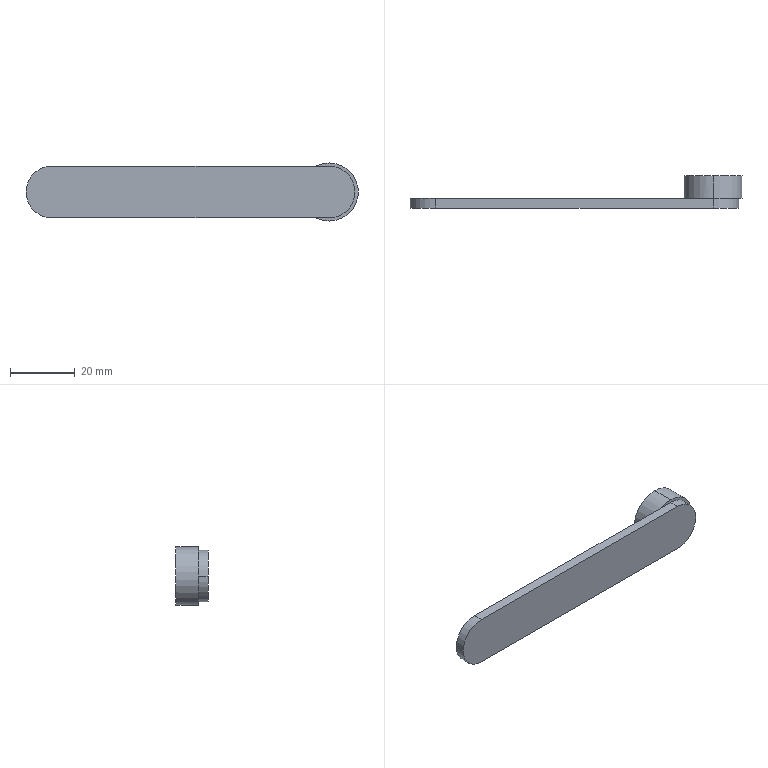Part | STEP file | 开关-3 | 1 solid | 12 faces | box 103 x 10 x 18 mm | volume 6512 mm3 | cylinder 6 | plane 6 | commonest cylinder face diameters 16 x4 18 x2
STEP:
#1=CARTESIAN_POINT('',(0.,0.,0.));
#2=DIRECTION('',(0.,0.,1.));
#3=DIRECTION('',(1.,0.,0.));
#4=AXIS2_PLACEMENT_3D('',#1,#2,#3);
#5=CARTESIAN_POINT('',(43.,10.,9.));
#6=VERTEX_POINT('',#5);
#7=CARTESIAN_POINT('',(43.,10.,-9.));
#8=VERTEX_POINT('',#7);
#9=CARTESIAN_POINT('',(43.,10.,0.));
#10=DIRECTION('',(0.,1.,0.));
#11=DIRECTION('',(0.,0.,1.));
#12=AXIS2_PLACEMENT_3D('',#9,#10,#11);
#13=CIRCLE('',#12,9.);
#14=CARTESIAN_POINT('',(43.,10.,0.));
#15=DIRECTION('',(0.,-1.,0.));
#16=DIRECTION('',(0.,0.,-1.));
#17=AXIS2_PLACEMENT_3D('',#14,#15,#16);
#18=CYLINDRICAL_SURFACE('',#17,9.);
#19=CARTESIAN_POINT('',(3.142,0.));
#20=DIRECTION('',(-1.,0.));
#21=VECTOR('',#20,1.);
#22=LINE('',#19,#21);
#23=(GEOMETRIC_REPRESENTATION_CONTEXT(2)PARAMETRIC_REPRESENTATION_CONTEXT()REPRESENTATION_CONTEXT('',''));
#24=DEFINITIONAL_REPRESENTATION('',(#22),#23);
#25=PCURVE('',#18,#24);
#26=CARTESIAN_POINT('',(43.,10.,0.));
#27=DIRECTION('',(0.,1.,0.));
#28=DIRECTION('',(0.,0.,1.));
#29=AXIS2_PLACEMENT_3D('',#26,#27,#28);
#30=PLANE('',#29);
#31=CARTESIAN_POINT('',(0.,0.));
#32=DIRECTION('',(1.,0.));
#33=AXIS2_PLACEMENT_2D('',#31,#32);
#34=CIRCLE('',#33,9.);
#35=(GEOMETRIC_REPRESENTATION_CONTEXT(2)PARAMETRIC_REPRESENTATION_CONTEXT()REPRESENTATION_CONTEXT('',''));
#36=DEFINITIONAL_REPRESENTATION('',(#34),#35);
#37=PCURVE('',#30,#36);
#38=SURFACE_CURVE('',#13,(#25,#37),.PCURVE_S1.);
#39=EDGE_CURVE('',#6,#8,#38,.T.);
#40=ORIENTED_EDGE('',*,*,#39,.F.);
#41=CARTESIAN_POINT('',(43.,3.,9.));
#42=VERTEX_POINT('',#41);
#43=CARTESIAN_POINT('',(43.,10.,9.));
#44=DIRECTION('',(0.,-1.,0.));
#45=VECTOR('',#44,1.);
#46=LINE('',#43,#45);
#47=CARTESIAN_POINT('',(3.142,0.));
#48=DIRECTION('',(0.,1.));
#49=VECTOR('',#48,1.);
#50=LINE('',#47,#49);
#51=(GEOMETRIC_REPRESENTATION_CONTEXT(2)PARAMETRIC_REPRESENTATION_CONTEXT()REPRESENTATION_CONTEXT('',''));
#52=DEFINITIONAL_REPRESENTATION('',(#50),#51);
#53=PCURVE('',#18,#52);
#54=CARTESIAN_POINT('',(43.,10.,0.));
#55=DIRECTION('',(0.,-1.,0.));
#56=DIRECTION('',(0.,0.,-1.));
#57=AXIS2_PLACEMENT_3D('',#54,#55,#56);
#58=CYLINDRICAL_SURFACE('',#57,9.);
#59=CARTESIAN_POINT('',(3.142,0.));
#60=DIRECTION('',(0.,1.));
#61=VECTOR('',#60,1.);
#62=LINE('',#59,#61);
#63=(GEOMETRIC_REPRESENTATION_CONTEXT(2)PARAMETRIC_REPRESENTATION_CONTEXT()REPRESENTATION_CONTEXT('',''));
#64=DEFINITIONAL_REPRESENTATION('',(#62),#63);
#65=PCURVE('',#58,#64);
#66=SURFACE_CURVE('',#46,(#53,#65),.PCURVE_S1.);
#67=EDGE_CURVE('',#6,#42,#66,.T.);
#68=ORIENTED_EDGE('',*,*,#67,.T.);
#69=CARTESIAN_POINT('',(43.,3.,-9.));
#70=VERTEX_POINT('',#69);
#71=CARTESIAN_POINT('',(43.,3.,0.));
#72=DIRECTION('',(0.,1.,0.));
#73=DIRECTION('',(0.,0.,1.));
#74=AXIS2_PLACEMENT_3D('',#71,#72,#73);
#75=CIRCLE('',#74,9.);
#76=CARTESIAN_POINT('',(3.142,7.));
#77=DIRECTION('',(-1.,0.));
#78=VECTOR('',#77,1.);
#79=LINE('',#76,#78);
#80=(GEOMETRIC_REPRESENTATION_CONTEXT(2)PARAMETRIC_REPRESENTATION_CONTEXT()REPRESENTATION_CONTEXT('',''));
#81=DEFINITIONAL_REPRESENTATION('',(#79),#80);
#82=PCURVE('',#18,#81);
#83=CARTESIAN_POINT('',(43.,3.,0.));
#84=DIRECTION('',(0.,1.,0.));
#85=DIRECTION('',(0.,0.,1.));
#86=AXIS2_PLACEMENT_3D('',#83,#84,#85);
#87=PLANE('',#86);
#88=CARTESIAN_POINT('',(0.,0.));
#89=DIRECTION('',(1.,0.));
#90=AXIS2_PLACEMENT_2D('',#88,#89);
#91=CIRCLE('',#90,9.);
#92=(GEOMETRIC_REPRESENTATION_CONTEXT(2)PARAMETRIC_REPRESENTATION_CONTEXT()REPRESENTATION_CONTEXT('',''));
#93=DEFINITIONAL_REPRESENTATION('',(#91),#92);
#94=PCURVE('',#87,#93);
#95=SURFACE_CURVE('',#75,(#82,#94),.PCURVE_S1.);
#96=EDGE_CURVE('',#42,#70,#95,.T.);
#97=ORIENTED_EDGE('',*,*,#96,.T.);
#98=CARTESIAN_POINT('',(43.,10.,-9.));
#99=DIRECTION('',(0.,-1.,0.));
#100=VECTOR('',#99,1.);
#101=LINE('',#98,#100);
#102=CARTESIAN_POINT('',(0.,0.));
#103=DIRECTION('',(0.,1.));
#104=VECTOR('',#103,1.);
#105=LINE('',#102,#104);
#106=(GEOMETRIC_REPRESENTATION_CONTEXT(2)PARAMETRIC_REPRESENTATION_CONTEXT()REPRESENTATION_CONTEXT('',''));
#107=DEFINITIONAL_REPRESENTATION('',(#105),#106);
#108=PCURVE('',#18,#107);
#109=CARTESIAN_POINT('',(6.283,0.));
#110=DIRECTION('',(0.,1.));
#111=VECTOR('',#110,1.);
#112=LINE('',#109,#111);
#113=(GEOMETRIC_REPRESENTATION_CONTEXT(2)PARAMETRIC_REPRESENTATION_CONTEXT()REPRESENTATION_CONTEXT('',''));
#114=DEFINITIONAL_REPRESENTATION('',(#112),#113);
#115=PCURVE('',#58,#114);
#116=SURFACE_CURVE('',#101,(#108,#115),.PCURVE_S1.);
#117=EDGE_CURVE('',#8,#70,#116,.T.);
#118=ORIENTED_EDGE('',*,*,#117,.F.);
#119=EDGE_LOOP('',(#40,#68,#97,#118));
#120=FACE_BOUND('',#119,.T.);
#121=ADVANCED_FACE('',(#120),#18,.T.);
#122=CARTESIAN_POINT('',(43.,0.,-8.));
#123=VERTEX_POINT('',#122);
#124=CARTESIAN_POINT('',(-43.,0.,-8.));
#125=VERTEX_POINT('',#124);
#126=CARTESIAN_POINT('',(-51.,0.,-8.));
#127=DIRECTION('',(-1.,0.,0.));
#128=VECTOR('',#127,1.);
#129=LINE('',#126,#128);
#130=CARTESIAN_POINT('',(-51.,3.,-8.));
#131=DIRECTION('',(0.,0.,1.));
#132=DIRECTION('',(1.,0.,0.));
#133=AXIS2_PLACEMENT_3D('',#130,#131,#132);
#134=PLANE('',#133);
#135=CARTESIAN_POINT('',(0.,-3.));
#136=DIRECTION('',(-1.,0.));
#137=VECTOR('',#136,1.);
#138=LINE('',#135,#137);
#139=(GEOMETRIC_REPRESENTATION_CONTEXT(2)PARAMETRIC_REPRESENTATION_CONTEXT()REPRESENTATION_CONTEXT('',''));
#140=DEFINITIONAL_REPRESENTATION('',(#138),#139);
#141=PCURVE('',#134,#140);
#142=CARTESIAN_POINT('',(0.,0.,0.));
#143=DIRECTION('',(0.,-1.,0.));
#144=DIRECTION('',(0.,0.,-1.));
#145=AXIS2_PLACEMENT_3D('',#142,#143,#144);
#146=PLANE('',#145);
#147=CARTESIAN_POINT('',(8.,-51.));
#148=DIRECTION('',(0.,-1.));
#149=VECTOR('',#148,1.);
#150=LINE('',#147,#149);
#151=(GEOMETRIC_REPRESENTATION_CONTEXT(2)PARAMETRIC_REPRESENTATION_CONTEXT()REPRESENTATION_CONTEXT('',''));
#152=DEFINITIONAL_REPRESENTATION('',(#150),#151);
#153=PCURVE('',#146,#152);
#154=SURFACE_CURVE('',#129,(#141,#153),.PCURVE_S1.);
#155=EDGE_CURVE('',#123,#125,#154,.T.);
#156=ORIENTED_EDGE('',*,*,#155,.T.);
#157=CARTESIAN_POINT('',(-43.,3.,-8.));
#158=VERTEX_POINT('',#157);
#159=CARTESIAN_POINT('',(-43.,3.,-8.));
#160=DIRECTION('',(0.,1.,0.));
#161=VECTOR('',#160,1.);
#162=LINE('',#159,#161);
#163=CARTESIAN_POINT('',(8.,0.));
#164=DIRECTION('',(0.,1.));
#165=VECTOR('',#164,1.);
#166=LINE('',#163,#165);
#167=(GEOMETRIC_REPRESENTATION_CONTEXT(2)PARAMETRIC_REPRESENTATION_CONTEXT()REPRESENTATION_CONTEXT('',''));
#168=DEFINITIONAL_REPRESENTATION('',(#166),#167);
#169=PCURVE('',#134,#168);
#170=CARTESIAN_POINT('',(-43.,3.,0.));
#171=DIRECTION('',(0.,-1.,0.));
#172=DIRECTION('',(0.,0.,-1.));
#173=AXIS2_PLACEMENT_3D('',#170,#171,#172);
#174=CYLINDRICAL_SURFACE('',#173,8.);
#175=CARTESIAN_POINT('',(6.283,0.));
#176=DIRECTION('',(0.,-1.));
#177=VECTOR('',#176,1.);
#178=LINE('',#175,#177);
#179=(GEOMETRIC_REPRESENTATION_CONTEXT(2)PARAMETRIC_REPRESENTATION_CONTEXT()REPRESENTATION_CONTEXT('',''));
#180=DEFINITIONAL_REPRESENTATION('',(#178),#179);
#181=PCURVE('',#174,#180);
#182=SURFACE_CURVE('',#162,(#169,#181),.PCURVE_S1.);
#183=EDGE_CURVE('',#125,#158,#182,.T.);
#184=ORIENTED_EDGE('',*,*,#183,.T.);
#185=CARTESIAN_POINT('',(38.877,3.,-8.));
#186=VERTEX_POINT('',#185);
#187=CARTESIAN_POINT('',(-51.,3.,-8.));
#188=DIRECTION('',(-1.,0.,0.));
#189=VECTOR('',#188,1.);
#190=LINE('',#187,#189);
#191=CARTESIAN_POINT('',(0.,0.));
#192=DIRECTION('',(-1.,0.));
#193=VECTOR('',#192,1.);
#194=LINE('',#191,#193);
#195=(GEOMETRIC_REPRESENTATION_CONTEXT(2)PARAMETRIC_REPRESENTATION_CONTEXT()REPRESENTATION_CONTEXT('',''));
#196=DEFINITIONAL_REPRESENTATION('',(#194),#195);
#197=PCURVE('',#134,#196);
#198=CARTESIAN_POINT('',(0.,3.,0.));
#199=DIRECTION('',(0.,-1.,0.));
#200=DIRECTION('',(0.,0.,-1.));
#201=AXIS2_PLACEMENT_3D('',#198,#199,#200);
#202=PLANE('',#201);
#203=CARTESIAN_POINT('',(8.,-51.));
#204=DIRECTION('',(0.,-1.));
#205=VECTOR('',#204,1.);
#206=LINE('',#203,#205);
#207=(GEOMETRIC_REPRESENTATION_CONTEXT(2)PARAMETRIC_REPRESENTATION_CONTEXT()REPRESENTATION_CONTEXT('',''));
#208=DEFINITIONAL_REPRESENTATION('',(#206),#207);
#209=PCURVE('',#202,#208);
#210=SURFACE_CURVE('',#190,(#197,#209),.PCURVE_S1.);
#211=EDGE_CURVE('',#186,#158,#210,.T.);
#212=ORIENTED_EDGE('',*,*,#211,.F.);
#213=CARTESIAN_POINT('',(43.,3.,-8.));
#214=VERTEX_POINT('',#213);
#215=CARTESIAN_POINT('',(-51.,3.,-8.));
#216=DIRECTION('',(-1.,0.,0.));
#217=VECTOR('',#216,1.);
#218=LINE('',#215,#217);
#219=CARTESIAN_POINT('',(0.,0.));
#220=DIRECTION('',(-1.,0.));
#221=VECTOR('',#220,1.);
#222=LINE('',#219,#221);
#223=(GEOMETRIC_REPRESENTATION_CONTEXT(2)PARAMETRIC_REPRESENTATION_CONTEXT()REPRESENTATION_CONTEXT('',''));
#224=DEFINITIONAL_REPRESENTATION('',(#222),#223);
#225=PCURVE('',#134,#224);
#226=CARTESIAN_POINT('',(-8.,-94.));
#227=DIRECTION('',(0.,-1.));
#228=VECTOR('',#227,1.);
#229=LINE('',#226,#228);
#230=(GEOMETRIC_REPRESENTATION_CONTEXT(2)PARAMETRIC_REPRESENTATION_CONTEXT()REPRESENTATION_CONTEXT('',''));
#231=DEFINITIONAL_REPRESENTATION('',(#229),#230);
#232=PCURVE('',#87,#231);
#233=SURFACE_CURVE('',#218,(#225,#232),.PCURVE_S1.);
#234=EDGE_CURVE('',#214,#186,#233,.T.);
#235=ORIENTED_EDGE('',*,*,#234,.F.);
#236=CARTESIAN_POINT('',(43.,3.,-8.));
#237=DIRECTION('',(0.,-1.,0.));
#238=VECTOR('',#237,1.);
#239=LINE('',#236,#238);
#240=CARTESIAN_POINT('',(94.,0.));
#241=DIRECTION('',(0.,-1.));
#242=VECTOR('',#241,1.);
#243=LINE('',#240,#242);
#244=(GEOMETRIC_REPRESENTATION_CONTEXT(2)PARAMETRIC_REPRESENTATION_CONTEXT()REPRESENTATION_CONTEXT('',''));
#245=DEFINITIONAL_REPRESENTATION('',(#243),#244);
#246=PCURVE('',#134,#245);
#247=CARTESIAN_POINT('',(43.,3.,0.));
#248=DIRECTION('',(0.,-1.,0.));
#249=DIRECTION('',(0.,0.,-1.));
#250=AXIS2_PLACEMENT_3D('',#247,#248,#249);
#251=CYLINDRICAL_SURFACE('',#250,8.);
#252=CARTESIAN_POINT('',(0.,0.));
#253=DIRECTION('',(0.,1.));
#254=VECTOR('',#253,1.);
#255=LINE('',#252,#254);
#256=(GEOMETRIC_REPRESENTATION_CONTEXT(2)PARAMETRIC_REPRESENTATION_CONTEXT()REPRESENTATION_CONTEXT('',''));
#257=DEFINITIONAL_REPRESENTATION('',(#255),#256);
#258=PCURVE('',#251,#257);
#259=SURFACE_CURVE('',#239,(#246,#258),.PCURVE_S1.);
#260=EDGE_CURVE('',#214,#123,#259,.T.);
#261=ORIENTED_EDGE('',*,*,#260,.T.);
#262=EDGE_LOOP('',(#156,#184,#212,#235,#261));
#263=FACE_BOUND('',#262,.T.);
#264=ADVANCED_FACE('',(#263),#134,.F.);
#265=CARTESIAN_POINT('',(-43.,3.,8.));
#266=VERTEX_POINT('',#265);
#267=CARTESIAN_POINT('',(38.877,3.,8.));
#268=VERTEX_POINT('',#267);
#269=CARTESIAN_POINT('',(-51.,3.,8.));
#270=DIRECTION('',(1.,0.,0.));
#271=VECTOR('',#270,1.);
#272=LINE('',#269,#271);
#273=CARTESIAN_POINT('',(-51.,3.,8.));
#274=DIRECTION('',(0.,0.,-1.));
#275=DIRECTION('',(-1.,0.,0.));
#276=AXIS2_PLACEMENT_3D('',#273,#274,#275);
#277=PLANE('',#276);
#278=CARTESIAN_POINT('',(0.,0.));
#279=DIRECTION('',(-1.,0.));
#280=VECTOR('',#279,1.);
#281=LINE('',#278,#280);
#282=(GEOMETRIC_REPRESENTATION_CONTEXT(2)PARAMETRIC_REPRESENTATION_CONTEXT()REPRESENTATION_CONTEXT('',''));
#283=DEFINITIONAL_REPRESENTATION('',(#281),#282);
#284=PCURVE('',#277,#283);
#285=CARTESIAN_POINT('',(-8.,-51.));
#286=DIRECTION('',(0.,1.));
#287=VECTOR('',#286,1.);
#288=LINE('',#285,#287);
#289=(GEOMETRIC_REPRESENTATION_CONTEXT(2)PARAMETRIC_REPRESENTATION_CONTEXT()REPRESENTATION_CONTEXT('',''));
#290=DEFINITIONAL_REPRESENTATION('',(#288),#289);
#291=PCURVE('',#202,#290);
#292=SURFACE_CURVE('',#272,(#284,#291),.PCURVE_S1.);
#293=EDGE_CURVE('',#266,#268,#292,.T.);
#294=ORIENTED_EDGE('',*,*,#293,.F.);
#295=CARTESIAN_POINT('',(-43.,0.,8.));
#296=VERTEX_POINT('',#295);
#297=CARTESIAN_POINT('',(-43.,3.,8.));
#298=DIRECTION('',(0.,-1.,0.));
#299=VECTOR('',#298,1.);
#300=LINE('',#297,#299);
#301=CARTESIAN_POINT('',(-8.,0.));
#302=DIRECTION('',(0.,-1.));
#303=VECTOR('',#302,1.);
#304=LINE('',#301,#303);
#305=(GEOMETRIC_REPRESENTATION_CONTEXT(2)PARAMETRIC_REPRESENTATION_CONTEXT()REPRESENTATION_CONTEXT('',''));
#306=DEFINITIONAL_REPRESENTATION('',(#304),#305);
#307=PCURVE('',#277,#306);
#308=CARTESIAN_POINT('',(-43.,3.,0.));
#309=DIRECTION('',(0.,-1.,0.));
#310=DIRECTION('',(0.,0.,-1.));
#311=AXIS2_PLACEMENT_3D('',#308,#309,#310);
#312=CYLINDRICAL_SURFACE('',#311,8.);
#313=CARTESIAN_POINT('',(3.142,0.));
#314=DIRECTION('',(0.,1.));
#315=VECTOR('',#314,1.);
#316=LINE('',#313,#315);
#317=(GEOMETRIC_REPRESENTATION_CONTEXT(2)PARAMETRIC_REPRESENTATION_CONTEXT()REPRESENTATION_CONTEXT('',''));
#318=DEFINITIONAL_REPRESENTATION('',(#316),#317);
#319=PCURVE('',#312,#318);
#320=SURFACE_CURVE('',#300,(#307,#319),.PCURVE_S1.);
#321=EDGE_CURVE('',#266,#296,#320,.T.);
#322=ORIENTED_EDGE('',*,*,#321,.T.);
#323=CARTESIAN_POINT('',(43.,0.,8.));
#324=VERTEX_POINT('',#323);
#325=CARTESIAN_POINT('',(-51.,0.,8.));
#326=DIRECTION('',(1.,0.,0.));
#327=VECTOR('',#326,1.);
#328=LINE('',#325,#327);
#329=CARTESIAN_POINT('',(0.,-3.));
#330=DIRECTION('',(-1.,0.));
#331=VECTOR('',#330,1.);
#332=LINE('',#329,#331);
#333=(GEOMETRIC_REPRESENTATION_CONTEXT(2)PARAMETRIC_REPRESENTATION_CONTEXT()REPRESENTATION_CONTEXT('',''));
#334=DEFINITIONAL_REPRESENTATION('',(#332),#333);
#335=PCURVE('',#277,#334);
#336=CARTESIAN_POINT('',(-8.,-51.));
#337=DIRECTION('',(0.,1.));
#338=VECTOR('',#337,1.);
#339=LINE('',#336,#338);
#340=(GEOMETRIC_REPRESENTATION_CONTEXT(2)PARAMETRIC_REPRESENTATION_CONTEXT()REPRESENTATION_CONTEXT('',''));
#341=DEFINITIONAL_REPRESENTATION('',(#339),#340);
#342=PCURVE('',#146,#341);
#343=SURFACE_CURVE('',#328,(#335,#342),.PCURVE_S1.);
#344=EDGE_CURVE('',#296,#324,#343,.T.);
#345=ORIENTED_EDGE('',*,*,#344,.T.);
#346=CARTESIAN_POINT('',(43.,3.,8.));
#347=VERTEX_POINT('',#346);
#348=CARTESIAN_POINT('',(43.,3.,8.));
#349=DIRECTION('',(0.,1.,0.));
#350=VECTOR('',#349,1.);
#351=LINE('',#348,#350);
#352=CARTESIAN_POINT('',(-94.,0.));
#353=DIRECTION('',(0.,1.));
#354=VECTOR('',#353,1.);
#355=LINE('',#352,#354);
#356=(GEOMETRIC_REPRESENTATION_CONTEXT(2)PARAMETRIC_REPRESENTATION_CONTEXT()REPRESENTATION_CONTEXT('',''));
#357=DEFINITIONAL_REPRESENTATION('',(#355),#356);
#358=PCURVE('',#277,#357);
#359=CARTESIAN_POINT('',(43.,3.,0.));
#360=DIRECTION('',(0.,-1.,0.));
#361=DIRECTION('',(0.,0.,-1.));
#362=AXIS2_PLACEMENT_3D('',#359,#360,#361);
#363=CYLINDRICAL_SURFACE('',#362,8.);
#364=CARTESIAN_POINT('',(3.142,0.));
#365=DIRECTION('',(0.,-1.));
#366=VECTOR('',#365,1.);
#367=LINE('',#364,#366);
#368=(GEOMETRIC_REPRESENTATION_CONTEXT(2)PARAMETRIC_REPRESENTATION_CONTEXT()REPRESENTATION_CONTEXT('',''));
#369=DEFINITIONAL_REPRESENTATION('',(#367),#368);
#370=PCURVE('',#363,#369);
#371=SURFACE_CURVE('',#351,(#358,#370),.PCURVE_S1.);
#372=EDGE_CURVE('',#324,#347,#371,.T.);
#373=ORIENTED_EDGE('',*,*,#372,.T.);
#374=CARTESIAN_POINT('',(-51.,3.,8.));
#375=DIRECTION('',(1.,0.,0.));
#376=VECTOR('',#375,1.);
#377=LINE('',#374,#376);
#378=CARTESIAN_POINT('',(0.,0.));
#379=DIRECTION('',(-1.,0.));
#380=VECTOR('',#379,1.);
#381=LINE('',#378,#380);
#382=(GEOMETRIC_REPRESENTATION_CONTEXT(2)PARAMETRIC_REPRESENTATION_CONTEXT()REPRESENTATION_CONTEXT('',''));
#383=DEFINITIONAL_REPRESENTATION('',(#381),#382);
#384=PCURVE('',#277,#383);
#385=CARTESIAN_POINT('',(8.,-94.));
#386=DIRECTION('',(0.,1.));
#387=VECTOR('',#386,1.);
#388=LINE('',#385,#387);
#389=(GEOMETRIC_REPRESENTATION_CONTEXT(2)PARAMETRIC_REPRESENTATION_CONTEXT()REPRESENTATION_CONTEXT('',''));
#390=DEFINITIONAL_REPRESENTATION('',(#388),#389);
#391=PCURVE('',#87,#390);
#392=SURFACE_CURVE('',#377,(#384,#391),.PCURVE_S1.);
#393=EDGE_CURVE('',#268,#347,#392,.T.);
#394=ORIENTED_EDGE('',*,*,#393,.F.);
#395=EDGE_LOOP('',(#294,#322,#345,#373,#394));
#396=FACE_BOUND('',#395,.T.);
#397=ADVANCED_FACE('',(#396),#277,.F.);
#398=CARTESIAN_POINT('',(43.,3.,0.));
#399=DIRECTION('',(0.,1.,0.));
#400=DIRECTION('',(0.,0.,1.));
#401=AXIS2_PLACEMENT_3D('',#398,#399,#400);
#402=CIRCLE('',#401,9.);
#403=CARTESIAN_POINT('',(-9.,43.));
#404=CARTESIAN_POINT('',(-9.,58.588));
#405=CARTESIAN_POINT('',(4.5,50.794));
#406=CARTESIAN_POINT('',(18.,43.));
#407=CARTESIAN_POINT('',(4.5,35.206));
#408=CARTESIAN_POINT('',(-9.,27.412));
#409=CARTESIAN_POINT('',(-9.,43.));
#410=(BOUNDED_CURVE()B_SPLINE_CURVE(2,(#403,#404,#405,#406,#407,#408,#409),.UNSPECIFIED.,.T.,.F.)B_SPLINE_CURVE_WITH_KNOTS((1,2,2,2,2,1),(-2.094,0.,2.094,4.189,6.283,8.378),.UNSPECIFIED.)CURVE()GEOMETRIC_REPRESENTATION_ITEM()RATIONAL_B_SPLINE_CURVE((1.,0.5,1.,0.5,1.,0.5,1.))REPRESENTATION_ITEM(''));
#411=(GEOMETRIC_REPRESENTATION_CONTEXT(2)PARAMETRIC_REPRESENTATION_CONTEXT()REPRESENTATION_CONTEXT('',''));
#412=DEFINITIONAL_REPRESENTATION('',(#410),#411);
#413=PCURVE('',#202,#412);
#414=CARTESIAN_POINT('',(9.425,7.));
#415=DIRECTION('',(-1.,0.));
#416=VECTOR('',#415,1.);
#417=LINE('',#414,#416);
#418=(GEOMETRIC_REPRESENTATION_CONTEXT(2)PARAMETRIC_REPRESENTATION_CONTEXT()REPRESENTATION_CONTEXT('',''));
#419=DEFINITIONAL_REPRESENTATION('',(#417),#418);
#420=PCURVE('',#58,#419);
#421=SURFACE_CURVE('',#402,(#413,#420),.PCURVE_S1.);
#422=EDGE_CURVE('',#186,#268,#421,.T.);
#423=ORIENTED_EDGE('',*,*,#422,.F.);
#424=ORIENTED_EDGE('',*,*,#211,.T.);
#425=CARTESIAN_POINT('',(-51.,3.,0.));
#426=VERTEX_POINT('',#425);
#427=CARTESIAN_POINT('',(-43.,3.,0.));
#428=DIRECTION('',(0.,1.,0.));
#429=DIRECTION('',(0.,0.,-1.));
#430=AXIS2_PLACEMENT_3D('',#427,#428,#429);
#431=CIRCLE('',#430,8.);
#432=CARTESIAN_POINT('',(8.,-43.));
#433=CARTESIAN_POINT('',(8.,-56.856));
#434=CARTESIAN_POINT('',(-4.,-49.928));
#435=CARTESIAN_POINT('',(-16.,-43.));
#436=CARTESIAN_POINT('',(-4.,-36.072));
#437=CARTESIAN_POINT('',(8.,-29.144));
#438=CARTESIAN_POINT('',(8.,-43.));
#439=(BOUNDED_CURVE()B_SPLINE_CURVE(2,(#432,#433,#434,#435,#436,#437,#438),.UNSPECIFIED.,.T.,.F.)B_SPLINE_CURVE_WITH_KNOTS((1,2,2,2,2,1),(-2.094,0.,2.094,4.189,6.283,8.378),.UNSPECIFIED.)CURVE()GEOMETRIC_REPRESENTATION_ITEM()RATIONAL_B_SPLINE_CURVE((1.,0.5,1.,0.5,1.,0.5,1.))REPRESENTATION_ITEM(''));
#440=(GEOMETRIC_REPRESENTATION_CONTEXT(2)PARAMETRIC_REPRESENTATION_CONTEXT()REPRESENTATION_CONTEXT('',''));
#441=DEFINITIONAL_REPRESENTATION('',(#439),#440);
#442=PCURVE('',#202,#441);
#443=CARTESIAN_POINT('',(6.283,0.));
#444=DIRECTION('',(-1.,0.));
#445=VECTOR('',#444,1.);
#446=LINE('',#443,#445);
#447=(GEOMETRIC_REPRESENTATION_CONTEXT(2)PARAMETRIC_REPRESENTATION_CONTEXT()REPRESENTATION_CONTEXT('',''));
#448=DEFINITIONAL_REPRESENTATION('',(#446),#447);
#449=PCURVE('',#174,#448);
#450=SURFACE_CURVE('',#431,(#442,#449),.PCURVE_S1.);
#451=EDGE_CURVE('',#158,#426,#450,.T.);
#452=ORIENTED_EDGE('',*,*,#451,.T.);
#453=CARTESIAN_POINT('',(-43.,3.,0.));
#454=DIRECTION('',(0.,1.,0.));
#455=DIRECTION('',(0.,0.,-1.));
#456=AXIS2_PLACEMENT_3D('',#453,#454,#455);
#457=CIRCLE('',#456,8.);
#458=CARTESIAN_POINT('',(8.,-43.));
#459=CARTESIAN_POINT('',(8.,-56.856));
#460=CARTESIAN_POINT('',(-4.,-49.928));
#461=CARTESIAN_POINT('',(-16.,-43.));
#462=CARTESIAN_POINT('',(-4.,-36.072));
#463=CARTESIAN_POINT('',(8.,-29.144));
#464=CARTESIAN_POINT('',(8.,-43.));
#465=(BOUNDED_CURVE()B_SPLINE_CURVE(2,(#458,#459,#460,#461,#462,#463,#464),.UNSPECIFIED.,.T.,.F.)B_SPLINE_CURVE_WITH_KNOTS((1,2,2,2,2,1),(-2.094,0.,2.094,4.189,6.283,8.378),.UNSPECIFIED.)CURVE()GEOMETRIC_REPRESENTATION_ITEM()RATIONAL_B_SPLINE_CURVE((1.,0.5,1.,0.5,1.,0.5,1.))REPRESENTATION_ITEM(''));
#466=(GEOMETRIC_REPRESENTATION_CONTEXT(2)PARAMETRIC_REPRESENTATION_CONTEXT()REPRESENTATION_CONTEXT('',''));
#467=DEFINITIONAL_REPRESENTATION('',(#465),#466);
#468=PCURVE('',#202,#467);
#469=CARTESIAN_POINT('',(6.283,0.));
#470=DIRECTION('',(-1.,0.));
#471=VECTOR('',#470,1.);
#472=LINE('',#469,#471);
#473=(GEOMETRIC_REPRESENTATION_CONTEXT(2)PARAMETRIC_REPRESENTATION_CONTEXT()REPRESENTATION_CONTEXT('',''));
#474=DEFINITIONAL_REPRESENTATION('',(#472),#473);
#475=PCURVE('',#312,#474);
#476=SURFACE_CURVE('',#457,(#468,#475),.PCURVE_S1.);
#477=EDGE_CURVE('',#426,#266,#476,.T.);
#478=ORIENTED_EDGE('',*,*,#477,.T.);
#479=ORIENTED_EDGE('',*,*,#293,.T.);
#480=EDGE_LOOP('',(#423,#424,#452,#478,#479));
#481=FACE_BOUND('',#480,.T.);
#482=ADVANCED_FACE('',(#481),#202,.F.);
#483=ORIENTED_EDGE('',*,*,#344,.F.);
#484=CARTESIAN_POINT('',(-51.,0.,0.));
#485=VERTEX_POINT('',#484);
#486=CARTESIAN_POINT('',(-43.,0.,0.));
#487=DIRECTION('',(0.,-1.,0.));
#488=DIRECTION('',(0.,0.,-1.));
#489=AXIS2_PLACEMENT_3D('',#486,#487,#488);
#490=CIRCLE('',#489,8.);
#491=CARTESIAN_POINT('',(0.,-43.));
#492=DIRECTION('',(1.,0.));
#493=AXIS2_PLACEMENT_2D('',#491,#492);
#494=CIRCLE('',#493,8.);
#495=(GEOMETRIC_REPRESENTATION_CONTEXT(2)PARAMETRIC_REPRESENTATION_CONTEXT()REPRESENTATION_CONTEXT('',''));
#496=DEFINITIONAL_REPRESENTATION('',(#494),#495);
#497=PCURVE('',#146,#496);
#498=CARTESIAN_POINT('',(0.,3.));
#499=DIRECTION('',(1.,0.));
#500=VECTOR('',#499,1.);
#501=LINE('',#498,#500);
#502=(GEOMETRIC_REPRESENTATION_CONTEXT(2)PARAMETRIC_REPRESENTATION_CONTEXT()REPRESENTATION_CONTEXT('',''));
#503=DEFINITIONAL_REPRESENTATION('',(#501),#502);
#504=PCURVE('',#312,#503);
#505=SURFACE_CURVE('',#490,(#497,#504),.PCURVE_S1.);
#506=EDGE_CURVE('',#296,#485,#505,.T.);
#507=ORIENTED_EDGE('',*,*,#506,.T.);
#508=CARTESIAN_POINT('',(-43.,0.,0.));
#509=DIRECTION('',(0.,-1.,0.));
#510=DIRECTION('',(0.,0.,-1.));
#511=AXIS2_PLACEMENT_3D('',#508,#509,#510);
#512=CIRCLE('',#511,8.);
#513=CARTESIAN_POINT('',(0.,-43.));
#514=DIRECTION('',(1.,0.));
#515=AXIS2_PLACEMENT_2D('',#513,#514);
#516=CIRCLE('',#515,8.);
#517=(GEOMETRIC_REPRESENTATION_CONTEXT(2)PARAMETRIC_REPRESENTATION_CONTEXT()REPRESENTATION_CONTEXT('',''));
#518=DEFINITIONAL_REPRESENTATION('',(#516),#517);
#519=PCURVE('',#146,#518);
#520=CARTESIAN_POINT('',(0.,3.));
#521=DIRECTION('',(1.,0.));
#522=VECTOR('',#521,1.);
#523=LINE('',#520,#522);
#524=(GEOMETRIC_REPRESENTATION_CONTEXT(2)PARAMETRIC_REPRESENTATION_CONTEXT()REPRESENTATION_CONTEXT('',''));
#525=DEFINITIONAL_REPRESENTATION('',(#523),#524);
#526=PCURVE('',#174,#525);
#527=SURFACE_CURVE('',#512,(#519,#526),.PCURVE_S1.);
#528=EDGE_CURVE('',#485,#125,#527,.T.);
#529=ORIENTED_EDGE('',*,*,#528,.T.);
#530=ORIENTED_EDGE('',*,*,#155,.F.);
#531=CARTESIAN_POINT('',(51.,0.,0.));
#532=VERTEX_POINT('',#531);
#533=CARTESIAN_POINT('',(43.,0.,0.));
#534=DIRECTION('',(0.,-1.,0.));
#535=DIRECTION('',(0.,0.,-1.));
#536=AXIS2_PLACEMENT_3D('',#533,#534,#535);
#537=CIRCLE('',#536,8.);
#538=CARTESIAN_POINT('',(0.,43.));
#539=DIRECTION('',(1.,0.));
#540=AXIS2_PLACEMENT_2D('',#538,#539);
#541=CIRCLE('',#540,8.);
#542=(GEOMETRIC_REPRESENTATION_CONTEXT(2)PARAMETRIC_REPRESENTATION_CONTEXT()REPRESENTATION_CONTEXT('',''));
#543=DEFINITIONAL_REPRESENTATION('',(#541),#542);
#544=PCURVE('',#146,#543);
#545=CARTESIAN_POINT('',(0.,3.));
#546=DIRECTION('',(1.,0.));
#547=VECTOR('',#546,1.);
#548=LINE('',#545,#547);
#549=(GEOMETRIC_REPRESENTATION_CONTEXT(2)PARAMETRIC_REPRESENTATION_CONTEXT()REPRESENTATION_CONTEXT('',''));
#550=DEFINITIONAL_REPRESENTATION('',(#548),#549);
#551=PCURVE('',#251,#550);
#552=SURFACE_CURVE('',#537,(#544,#551),.PCURVE_S1.);
#553=EDGE_CURVE('',#123,#532,#552,.T.);
#554=ORIENTED_EDGE('',*,*,#553,.T.);
#555=CARTESIAN_POINT('',(43.,0.,0.));
#556=DIRECTION('',(0.,-1.,0.));
#557=DIRECTION('',(0.,0.,-1.));
#558=AXIS2_PLACEMENT_3D('',#555,#556,#557);
#559=CIRCLE('',#558,8.);
#560=CARTESIAN_POINT('',(0.,43.));
#561=DIRECTION('',(1.,0.));
#562=AXIS2_PLACEMENT_2D('',#560,#561);
#563=CIRCLE('',#562,8.);
#564=(GEOMETRIC_REPRESENTATION_CONTEXT(2)PARAMETRIC_REPRESENTATION_CONTEXT()REPRESENTATION_CONTEXT('',''));
#565=DEFINITIONAL_REPRESENTATION('',(#563),#564);
#566=PCURVE('',#146,#565);
#567=CARTESIAN_POINT('',(0.,3.));
#568=DIRECTION('',(1.,0.));
#569=VECTOR('',#568,1.);
#570=LINE('',#567,#569);
#571=(GEOMETRIC_REPRESENTATION_CONTEXT(2)PARAMETRIC_REPRESENTATION_CONTEXT()REPRESENTATION_CONTEXT('',''));
#572=DEFINITIONAL_REPRESENTATION('',(#570),#571);
#573=PCURVE('',#363,#572);
#574=SURFACE_CURVE('',#559,(#566,#573),.PCURVE_S1.);
#575=EDGE_CURVE('',#532,#324,#574,.T.);
#576=ORIENTED_EDGE('',*,*,#575,.T.);
#577=EDGE_LOOP('',(#483,#507,#529,#530,#554,#576));
#578=FACE_BOUND('',#577,.T.);
#579=ADVANCED_FACE('',(#578),#146,.T.);
#580=CARTESIAN_POINT('',(-51.,3.,0.));
#581=DIRECTION('',(0.,-1.,0.));
#582=VECTOR('',#581,1.);
#583=LINE('',#580,#582);
#584=CARTESIAN_POINT('',(4.712,0.));
#585=DIRECTION('',(0.,1.));
#586=VECTOR('',#585,1.);
#587=LINE('',#584,#586);
#588=(GEOMETRIC_REPRESENTATION_CONTEXT(2)PARAMETRIC_REPRESENTATION_CONTEXT()REPRESENTATION_CONTEXT('',''));
#589=DEFINITIONAL_REPRESENTATION('',(#587),#588);
#590=PCURVE('',#174,#589);
#591=CARTESIAN_POINT('',(4.712,0.));
#592=DIRECTION('',(0.,1.));
#593=VECTOR('',#592,1.);
#594=LINE('',#591,#593);
#595=(GEOMETRIC_REPRESENTATION_CONTEXT(2)PARAMETRIC_REPRESENTATION_CONTEXT()REPRESENTATION_CONTEXT('',''));
#596=DEFINITIONAL_REPRESENTATION('',(#594),#595);
#597=PCURVE('',#312,#596);
#598=SURFACE_CURVE('',#583,(#590,#597),.PCURVE_S1.);
#599=EDGE_CURVE('',#426,#485,#598,.T.);
#600=ORIENTED_EDGE('',*,*,#599,.F.);
#601=ORIENTED_EDGE('',*,*,#451,.F.);
#602=ORIENTED_EDGE('',*,*,#183,.F.);
#603=ORIENTED_EDGE('',*,*,#528,.F.);
#604=EDGE_LOOP('',(#600,#601,#602,#603));
#605=FACE_BOUND('',#604,.T.);
#606=ADVANCED_FACE('',(#605),#174,.T.);
#607=ORIENTED_EDGE('',*,*,#477,.F.);
#608=ORIENTED_EDGE('',*,*,#599,.T.);
#609=ORIENTED_EDGE('',*,*,#506,.F.);
#610=ORIENTED_EDGE('',*,*,#321,.F.);
#611=EDGE_LOOP('',(#607,#608,#609,#610));
#612=FACE_BOUND('',#611,.T.);
#613=ADVANCED_FACE('',(#612),#312,.T.);
#614=CARTESIAN_POINT('',(51.,3.,0.));
#615=VERTEX_POINT('',#614);
#616=CARTESIAN_POINT('',(51.,3.,0.));
#617=DIRECTION('',(0.,-1.,0.));
#618=VECTOR('',#617,1.);
#619=LINE('',#616,#618);
#620=CARTESIAN_POINT('',(1.571,0.));
#621=DIRECTION('',(0.,1.));
#622=VECTOR('',#621,1.);
#623=LINE('',#620,#622);
#624=(GEOMETRIC_REPRESENTATION_CONTEXT(2)PARAMETRIC_REPRESENTATION_CONTEXT()REPRESENTATION_CONTEXT('',''));
#625=DEFINITIONAL_REPRESENTATION('',(#623),#624);
#626=PCURVE('',#363,#625);
#627=CARTESIAN_POINT('',(1.571,0.));
#628=DIRECTION('',(0.,1.));
#629=VECTOR('',#628,1.);
#630=LINE('',#627,#629);
#631=(GEOMETRIC_REPRESENTATION_CONTEXT(2)PARAMETRIC_REPRESENTATION_CONTEXT()REPRESENTATION_CONTEXT('',''));
#632=DEFINITIONAL_REPRESENTATION('',(#630),#631);
#633=PCURVE('',#251,#632);
#634=SURFACE_CURVE('',#619,(#626,#633),.PCURVE_S1.);
#635=EDGE_CURVE('',#615,#532,#634,.T.);
#636=ORIENTED_EDGE('',*,*,#635,.F.);
#637=CARTESIAN_POINT('',(43.,3.,0.));
#638=DIRECTION('',(0.,1.,0.));
#639=DIRECTION('',(0.,0.,-1.));
#640=AXIS2_PLACEMENT_3D('',#637,#638,#639);
#641=CIRCLE('',#640,8.);
#642=CARTESIAN_POINT('',(6.283,0.));
#643=DIRECTION('',(-1.,0.));
#644=VECTOR('',#643,1.);
#645=LINE('',#642,#644);
#646=(GEOMETRIC_REPRESENTATION_CONTEXT(2)PARAMETRIC_REPRESENTATION_CONTEXT()REPRESENTATION_CONTEXT('',''));
#647=DEFINITIONAL_REPRESENTATION('',(#645),#646);
#648=PCURVE('',#363,#647);
#649=CARTESIAN_POINT('',(0.,0.));
#650=DIRECTION('',(-1.,0.));
#651=AXIS2_PLACEMENT_2D('',#649,#650);
#652=CIRCLE('',#651,8.);
#653=(GEOMETRIC_REPRESENTATION_CONTEXT(2)PARAMETRIC_REPRESENTATION_CONTEXT()REPRESENTATION_CONTEXT('',''));
#654=DEFINITIONAL_REPRESENTATION('',(#652),#653);
#655=PCURVE('',#87,#654);
#656=SURFACE_CURVE('',#641,(#648,#655),.PCURVE_S1.);
#657=EDGE_CURVE('',#347,#615,#656,.T.);
#658=ORIENTED_EDGE('',*,*,#657,.F.);
#659=ORIENTED_EDGE('',*,*,#372,.F.);
#660=ORIENTED_EDGE('',*,*,#575,.F.);
#661=EDGE_LOOP('',(#636,#658,#659,#660));
#662=FACE_BOUND('',#661,.T.);
#663=ADVANCED_FACE('',(#662),#363,.T.);
#664=CARTESIAN_POINT('',(43.,3.,0.));
#665=DIRECTION('',(0.,1.,0.));
#666=DIRECTION('',(0.,0.,-1.));
#667=AXIS2_PLACEMENT_3D('',#664,#665,#666);
#668=CIRCLE('',#667,8.);
#669=CARTESIAN_POINT('',(6.283,0.));
#670=DIRECTION('',(-1.,0.));
#671=VECTOR('',#670,1.);
#672=LINE('',#669,#671);
#673=(GEOMETRIC_REPRESENTATION_CONTEXT(2)PARAMETRIC_REPRESENTATION_CONTEXT()REPRESENTATION_CONTEXT('',''));
#674=DEFINITIONAL_REPRESENTATION('',(#672),#673);
#675=PCURVE('',#251,#674);
#676=CARTESIAN_POINT('',(0.,0.));
#677=DIRECTION('',(-1.,0.));
#678=AXIS2_PLACEMENT_2D('',#676,#677);
#679=CIRCLE('',#678,8.);
#680=(GEOMETRIC_REPRESENTATION_CONTEXT(2)PARAMETRIC_REPRESENTATION_CONTEXT()REPRESENTATION_CONTEXT('',''));
#681=DEFINITIONAL_REPRESENTATION('',(#679),#680);
#682=PCURVE('',#87,#681);
#683=SURFACE_CURVE('',#668,(#675,#682),.PCURVE_S1.);
#684=EDGE_CURVE('',#615,#214,#683,.T.);
#685=ORIENTED_EDGE('',*,*,#684,.F.);
#686=ORIENTED_EDGE('',*,*,#635,.T.);
#687=ORIENTED_EDGE('',*,*,#553,.F.);
#688=ORIENTED_EDGE('',*,*,#260,.F.);
#689=EDGE_LOOP('',(#685,#686,#687,#688));
#690=FACE_BOUND('',#689,.T.);
#691=ADVANCED_FACE('',(#690),#251,.T.);
#692=CARTESIAN_POINT('',(43.,3.,0.));
#693=DIRECTION('',(0.,1.,0.));
#694=DIRECTION('',(0.,0.,1.));
#695=AXIS2_PLACEMENT_3D('',#692,#693,#694);
#696=CIRCLE('',#695,9.);
#697=CARTESIAN_POINT('',(0.,0.));
#698=DIRECTION('',(1.,0.));
#699=AXIS2_PLACEMENT_2D('',#697,#698);
#700=CIRCLE('',#699,9.);
#701=(GEOMETRIC_REPRESENTATION_CONTEXT(2)PARAMETRIC_REPRESENTATION_CONTEXT()REPRESENTATION_CONTEXT('',''));
#702=DEFINITIONAL_REPRESENTATION('',(#700),#701);
#703=PCURVE('',#87,#702);
#704=CARTESIAN_POINT('',(9.425,7.));
#705=DIRECTION('',(-1.,0.));
#706=VECTOR('',#705,1.);
#707=LINE('',#704,#706);
#708=(GEOMETRIC_REPRESENTATION_CONTEXT(2)PARAMETRIC_REPRESENTATION_CONTEXT()REPRESENTATION_CONTEXT('',''));
#709=DEFINITIONAL_REPRESENTATION('',(#707),#708);
#710=PCURVE('',#58,#709);
#711=SURFACE_CURVE('',#696,(#703,#710),.PCURVE_S1.);
#712=EDGE_CURVE('',#268,#42,#711,.T.);
#713=ORIENTED_EDGE('',*,*,#712,.F.);
#714=ORIENTED_EDGE('',*,*,#393,.T.);
#715=ORIENTED_EDGE('',*,*,#657,.T.);
#716=ORIENTED_EDGE('',*,*,#684,.T.);
#717=ORIENTED_EDGE('',*,*,#234,.T.);
#718=CARTESIAN_POINT('',(43.,3.,0.));
#719=DIRECTION('',(0.,1.,0.));
#720=DIRECTION('',(0.,0.,1.));
#721=AXIS2_PLACEMENT_3D('',#718,#719,#720);
#722=CIRCLE('',#721,9.);
#723=CARTESIAN_POINT('',(0.,0.));
#724=DIRECTION('',(1.,0.));
#725=AXIS2_PLACEMENT_2D('',#723,#724);
#726=CIRCLE('',#725,9.);
#727=(GEOMETRIC_REPRESENTATION_CONTEXT(2)PARAMETRIC_REPRESENTATION_CONTEXT()REPRESENTATION_CONTEXT('',''));
#728=DEFINITIONAL_REPRESENTATION('',(#726),#727);
#729=PCURVE('',#87,#728);
#730=CARTESIAN_POINT('',(9.425,7.));
#731=DIRECTION('',(-1.,0.));
#732=VECTOR('',#731,1.);
#733=LINE('',#730,#732);
#734=(GEOMETRIC_REPRESENTATION_CONTEXT(2)PARAMETRIC_REPRESENTATION_CONTEXT()REPRESENTATION_CONTEXT('',''));
#735=DEFINITIONAL_REPRESENTATION('',(#733),#734);
#736=PCURVE('',#58,#735);
#737=SURFACE_CURVE('',#722,(#729,#736),.PCURVE_S1.);
#738=EDGE_CURVE('',#70,#186,#737,.T.);
#739=ORIENTED_EDGE('',*,*,#738,.F.);
#740=ORIENTED_EDGE('',*,*,#96,.F.);
#741=EDGE_LOOP('',(#713,#714,#715,#716,#717,#739,#740));
#742=FACE_BOUND('',#741,.T.);
#743=ADVANCED_FACE('',(#742),#87,.F.);
#744=ORIENTED_EDGE('',*,*,#67,.F.);
#745=CARTESIAN_POINT('',(43.,10.,0.));
#746=DIRECTION('',(0.,1.,0.));
#747=DIRECTION('',(0.,0.,1.));
#748=AXIS2_PLACEMENT_3D('',#745,#746,#747);
#749=CIRCLE('',#748,9.);
#750=CARTESIAN_POINT('',(9.425,0.));
#751=DIRECTION('',(-1.,0.));
#752=VECTOR('',#751,1.);
#753=LINE('',#750,#752);
#754=(GEOMETRIC_REPRESENTATION_CONTEXT(2)PARAMETRIC_REPRESENTATION_CONTEXT()REPRESENTATION_CONTEXT('',''));
#755=DEFINITIONAL_REPRESENTATION('',(#753),#754);
#756=PCURVE('',#58,#755);
#757=CARTESIAN_POINT('',(0.,0.));
#758=DIRECTION('',(1.,0.));
#759=AXIS2_PLACEMENT_2D('',#757,#758);
#760=CIRCLE('',#759,9.);
#761=(GEOMETRIC_REPRESENTATION_CONTEXT(2)PARAMETRIC_REPRESENTATION_CONTEXT()REPRESENTATION_CONTEXT('',''));
#762=DEFINITIONAL_REPRESENTATION('',(#760),#761);
#763=PCURVE('',#30,#762);
#764=SURFACE_CURVE('',#749,(#756,#763),.PCURVE_S1.);
#765=EDGE_CURVE('',#8,#6,#764,.T.);
#766=ORIENTED_EDGE('',*,*,#765,.F.);
#767=ORIENTED_EDGE('',*,*,#117,.T.);
#768=ORIENTED_EDGE('',*,*,#738,.T.);
#769=ORIENTED_EDGE('',*,*,#422,.T.);
#770=ORIENTED_EDGE('',*,*,#712,.T.);
#771=EDGE_LOOP('',(#744,#766,#767,#768,#769,#770));
#772=FACE_BOUND('',#771,.T.);
#773=ADVANCED_FACE('',(#772),#58,.T.);
#774=ORIENTED_EDGE('',*,*,#765,.T.);
#775=ORIENTED_EDGE('',*,*,#39,.T.);
#776=EDGE_LOOP('',(#774,#775));
#777=FACE_BOUND('',#776,.T.);
#778=ADVANCED_FACE('',(#777),#30,.T.);
#779=CLOSED_SHELL('',(#121,#264,#397,#482,#579,#606,#613,#663,#691,#743,#773,#778));
#780=MANIFOLD_SOLID_BREP('',#779);
#781=(LENGTH_UNIT()NAMED_UNIT(*)SI_UNIT(.MILLI.,.METRE.));
#782=UNCERTAINTY_MEASURE_WITH_UNIT(LENGTH_MEASURE(0.0000001),#781,'','');
#783=(NAMED_UNIT(*)PLANE_ANGLE_UNIT()SI_UNIT($,.RADIAN.));
#784=(NAMED_UNIT(*)SI_UNIT($,.STERADIAN.)SOLID_ANGLE_UNIT());
#785=(GEOMETRIC_REPRESENTATION_CONTEXT(3)GLOBAL_UNCERTAINTY_ASSIGNED_CONTEXT((#782))GLOBAL_UNIT_ASSIGNED_CONTEXT((#781,#783,#784))REPRESENTATION_CONTEXT('',''));
#786=ADVANCED_BREP_SHAPE_REPRESENTATION('',(#4,#780),#785);